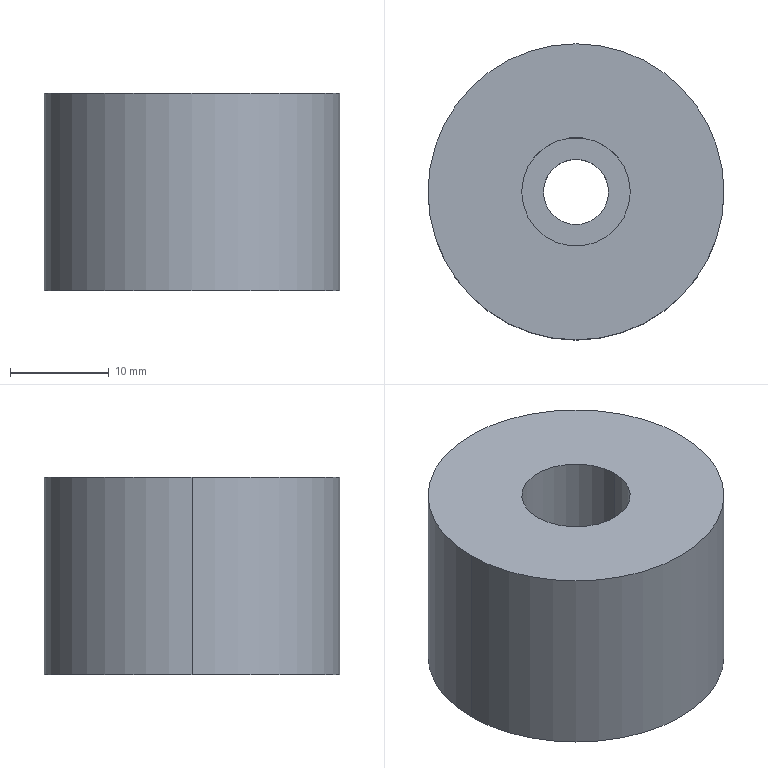Part | SolidWorks | features BaseBody 1 | 1 solid | 9 faces | box 30 x 30 x 20 mm | volume 12966 mm3 | cylinder 6 | plane 3 | commonest cylinder face diameters 6.6 x2 11 x2 30 x2
STEP:
#1=CARTESIAN_POINT('',(-15.,0.,20.));
#2=VERTEX_POINT('',#1);
#3=CARTESIAN_POINT('',(15.,0.,20.));
#4=VERTEX_POINT('',#3);
#5=CARTESIAN_POINT('',(0.,0.,20.));
#6=DIRECTION('',(0.,0.,-1.));
#7=DIRECTION('',(-1.,0.,0.));
#8=AXIS2_PLACEMENT_3D('',#5,#6,#7);
#9=CIRCLE('',#8,15.);
#10=EDGE_CURVE('',#2,#4,#9,.T.);
#11=ORIENTED_EDGE('',*,*,#10,.T.);
#12=CARTESIAN_POINT('',(15.,0.,0.));
#13=VERTEX_POINT('',#12);
#14=CARTESIAN_POINT('',(15.,0.,20.));
#15=DIRECTION('',(0.,0.,-1.));
#16=VECTOR('',#15,1000.);
#17=LINE('',#14,#16);
#18=EDGE_CURVE('',#4,#13,#17,.T.);
#19=ORIENTED_EDGE('',*,*,#18,.T.);
#20=CARTESIAN_POINT('',(-15.,0.,0.));
#21=VERTEX_POINT('',#20);
#22=CARTESIAN_POINT('',(0.,0.,0.));
#23=DIRECTION('',(0.,0.,1.));
#24=DIRECTION('',(-1.,0.,0.));
#25=AXIS2_PLACEMENT_3D('',#22,#23,#24);
#26=CIRCLE('',#25,15.);
#27=EDGE_CURVE('',#13,#21,#26,.T.);
#28=ORIENTED_EDGE('',*,*,#27,.T.);
#29=CARTESIAN_POINT('',(-15.,0.,20.));
#30=DIRECTION('',(0.,0.,-1.));
#31=VECTOR('',#30,1000.);
#32=LINE('',#29,#31);
#33=EDGE_CURVE('',#2,#21,#32,.T.);
#34=ORIENTED_EDGE('',*,*,#33,.F.);
#35=EDGE_LOOP('',(#11,#19,#28,#34));
#36=FACE_OUTER_BOUND('',#35,.T.);
#37=CARTESIAN_POINT('',(0.,0.,20.));
#38=DIRECTION('',(0.,0.,-1.));
#39=DIRECTION('',(-1.,0.,0.));
#40=AXIS2_PLACEMENT_3D('',#37,#38,#39);
#41=CYLINDRICAL_SURFACE('',#40,15.);
#42=ADVANCED_FACE('',(#36),#41,.T.);
#43=CARTESIAN_POINT('',(3.3,0.,0.));
#44=VERTEX_POINT('',#43);
#45=CARTESIAN_POINT('',(-3.3,0.,0.));
#46=VERTEX_POINT('',#45);
#47=CARTESIAN_POINT('',(0.,0.,0.));
#48=DIRECTION('',(0.,0.,-1.));
#49=DIRECTION('',(1.,0.,0.));
#50=AXIS2_PLACEMENT_3D('',#47,#48,#49);
#51=CIRCLE('',#50,3.3);
#52=EDGE_CURVE('',#44,#46,#51,.T.);
#53=ORIENTED_EDGE('',*,*,#52,.T.);
#54=CARTESIAN_POINT('',(-3.3,0.,12.));
#55=VERTEX_POINT('',#54);
#56=CARTESIAN_POINT('',(-3.3,0.,20.));
#57=DIRECTION('',(0.,0.,1.));
#58=VECTOR('',#57,1000.);
#59=LINE('',#56,#58);
#60=EDGE_CURVE('',#46,#55,#59,.T.);
#61=ORIENTED_EDGE('',*,*,#60,.T.);
#62=CARTESIAN_POINT('',(3.3,0.,12.));
#63=VERTEX_POINT('',#62);
#64=CARTESIAN_POINT('',(0.,0.,12.));
#65=DIRECTION('',(0.,0.,-1.));
#66=DIRECTION('',(1.,0.,0.));
#67=AXIS2_PLACEMENT_3D('',#64,#65,#66);
#68=CIRCLE('',#67,3.3);
#69=EDGE_CURVE('',#63,#55,#68,.T.);
#70=ORIENTED_EDGE('',*,*,#69,.F.);
#71=CARTESIAN_POINT('',(3.3,0.,20.));
#72=DIRECTION('',(0.,0.,1.));
#73=VECTOR('',#72,1000.);
#74=LINE('',#71,#73);
#75=EDGE_CURVE('',#44,#63,#74,.T.);
#76=ORIENTED_EDGE('',*,*,#75,.F.);
#77=EDGE_LOOP('',(#53,#61,#70,#76));
#78=FACE_OUTER_BOUND('',#77,.T.);
#79=CARTESIAN_POINT('',(0.,0.,20.));
#80=DIRECTION('',(0.,0.,1.));
#81=DIRECTION('',(1.,0.,0.));
#82=AXIS2_PLACEMENT_3D('',#79,#80,#81);
#83=CYLINDRICAL_SURFACE('',#82,3.3);
#84=ADVANCED_FACE('',(#78),#83,.F.);
#85=CARTESIAN_POINT('',(-5.5,0.,12.));
#86=VERTEX_POINT('',#85);
#87=CARTESIAN_POINT('',(5.5,0.,12.));
#88=VERTEX_POINT('',#87);
#89=CARTESIAN_POINT('',(0.,0.,12.));
#90=DIRECTION('',(0.,0.,1.));
#91=DIRECTION('',(1.,0.,0.));
#92=AXIS2_PLACEMENT_3D('',#89,#90,#91);
#93=CIRCLE('',#92,5.5);
#94=EDGE_CURVE('',#86,#88,#93,.T.);
#95=ORIENTED_EDGE('',*,*,#94,.F.);
#96=CARTESIAN_POINT('',(-5.5,0.,20.));
#97=VERTEX_POINT('',#96);
#98=CARTESIAN_POINT('',(-5.5,0.,20.));
#99=DIRECTION('',(0.,0.,1.));
#100=VECTOR('',#99,1000.);
#101=LINE('',#98,#100);
#102=EDGE_CURVE('',#86,#97,#101,.T.);
#103=ORIENTED_EDGE('',*,*,#102,.T.);
#104=CARTESIAN_POINT('',(5.5,0.,20.));
#105=VERTEX_POINT('',#104);
#106=CARTESIAN_POINT('',(0.,0.,20.));
#107=DIRECTION('',(0.,0.,-1.));
#108=DIRECTION('',(1.,0.,0.));
#109=AXIS2_PLACEMENT_3D('',#106,#107,#108);
#110=CIRCLE('',#109,5.5);
#111=EDGE_CURVE('',#105,#97,#110,.T.);
#112=ORIENTED_EDGE('',*,*,#111,.F.);
#113=CARTESIAN_POINT('',(5.5,0.,20.));
#114=DIRECTION('',(0.,0.,1.));
#115=VECTOR('',#114,1000.);
#116=LINE('',#113,#115);
#117=EDGE_CURVE('',#88,#105,#116,.T.);
#118=ORIENTED_EDGE('',*,*,#117,.F.);
#119=EDGE_LOOP('',(#95,#103,#112,#118));
#120=FACE_OUTER_BOUND('',#119,.T.);
#121=CARTESIAN_POINT('',(0.,0.,20.));
#122=DIRECTION('',(0.,0.,1.));
#123=DIRECTION('',(1.,0.,0.));
#124=AXIS2_PLACEMENT_3D('',#121,#122,#123);
#125=CYLINDRICAL_SURFACE('',#124,5.5);
#126=ADVANCED_FACE('',(#120),#125,.F.);
#127=ORIENTED_EDGE('',*,*,#18,.F.);
#128=CARTESIAN_POINT('',(0.,0.,20.));
#129=DIRECTION('',(0.,0.,-1.));
#130=DIRECTION('',(-1.,0.,0.));
#131=AXIS2_PLACEMENT_3D('',#128,#129,#130);
#132=CIRCLE('',#131,15.);
#133=EDGE_CURVE('',#4,#2,#132,.T.);
#134=ORIENTED_EDGE('',*,*,#133,.T.);
#135=ORIENTED_EDGE('',*,*,#33,.T.);
#136=CARTESIAN_POINT('',(0.,0.,0.));
#137=DIRECTION('',(0.,0.,1.));
#138=DIRECTION('',(-1.,0.,0.));
#139=AXIS2_PLACEMENT_3D('',#136,#137,#138);
#140=CIRCLE('',#139,15.);
#141=EDGE_CURVE('',#21,#13,#140,.T.);
#142=ORIENTED_EDGE('',*,*,#141,.T.);
#143=EDGE_LOOP('',(#127,#134,#135,#142));
#144=FACE_OUTER_BOUND('',#143,.T.);
#145=CARTESIAN_POINT('',(0.,0.,20.));
#146=DIRECTION('',(0.,0.,-1.));
#147=DIRECTION('',(-1.,0.,0.));
#148=AXIS2_PLACEMENT_3D('',#145,#146,#147);
#149=CYLINDRICAL_SURFACE('',#148,15.);
#150=ADVANCED_FACE('',(#144),#149,.T.);
#151=ORIENTED_EDGE('',*,*,#141,.F.);
#152=ORIENTED_EDGE('',*,*,#27,.F.);
#153=EDGE_LOOP('',(#151,#152));
#154=FACE_OUTER_BOUND('',#153,.T.);
#155=ORIENTED_EDGE('',*,*,#52,.F.);
#156=CARTESIAN_POINT('',(0.,0.,0.));
#157=DIRECTION('',(0.,0.,-1.));
#158=DIRECTION('',(1.,0.,0.));
#159=AXIS2_PLACEMENT_3D('',#156,#157,#158);
#160=CIRCLE('',#159,3.3);
#161=EDGE_CURVE('',#46,#44,#160,.T.);
#162=ORIENTED_EDGE('',*,*,#161,.F.);
#163=EDGE_LOOP('',(#155,#162));
#164=FACE_BOUND('',#163,.T.);
#165=CARTESIAN_POINT('',(0.,0.,0.));
#166=DIRECTION('',(0.,0.,1.));
#167=DIRECTION('',(1.,0.,0.));
#168=AXIS2_PLACEMENT_3D('',#165,#166,#167);
#169=PLANE('',#168);
#170=ADVANCED_FACE('',(#154,#164),#169,.F.);
#171=ORIENTED_EDGE('',*,*,#10,.F.);
#172=ORIENTED_EDGE('',*,*,#133,.F.);
#173=EDGE_LOOP('',(#171,#172));
#174=FACE_OUTER_BOUND('',#173,.T.);
#175=ORIENTED_EDGE('',*,*,#111,.T.);
#176=CARTESIAN_POINT('',(0.,0.,20.));
#177=DIRECTION('',(0.,0.,-1.));
#178=DIRECTION('',(1.,0.,0.));
#179=AXIS2_PLACEMENT_3D('',#176,#177,#178);
#180=CIRCLE('',#179,5.5);
#181=EDGE_CURVE('',#97,#105,#180,.T.);
#182=ORIENTED_EDGE('',*,*,#181,.T.);
#183=EDGE_LOOP('',(#175,#182));
#184=FACE_BOUND('',#183,.T.);
#185=CARTESIAN_POINT('',(0.,0.,20.));
#186=DIRECTION('',(0.,0.,1.));
#187=DIRECTION('',(1.,0.,0.));
#188=AXIS2_PLACEMENT_3D('',#185,#186,#187);
#189=PLANE('',#188);
#190=ADVANCED_FACE('',(#174,#184),#189,.T.);
#191=ORIENTED_EDGE('',*,*,#60,.F.);
#192=ORIENTED_EDGE('',*,*,#161,.T.);
#193=ORIENTED_EDGE('',*,*,#75,.T.);
#194=CARTESIAN_POINT('',(0.,0.,12.));
#195=DIRECTION('',(0.,0.,-1.));
#196=DIRECTION('',(1.,0.,0.));
#197=AXIS2_PLACEMENT_3D('',#194,#195,#196);
#198=CIRCLE('',#197,3.3);
#199=EDGE_CURVE('',#55,#63,#198,.T.);
#200=ORIENTED_EDGE('',*,*,#199,.F.);
#201=EDGE_LOOP('',(#191,#192,#193,#200));
#202=FACE_OUTER_BOUND('',#201,.T.);
#203=CARTESIAN_POINT('',(0.,0.,20.));
#204=DIRECTION('',(0.,0.,1.));
#205=DIRECTION('',(1.,0.,0.));
#206=AXIS2_PLACEMENT_3D('',#203,#204,#205);
#207=CYLINDRICAL_SURFACE('',#206,3.3);
#208=ADVANCED_FACE('',(#202),#207,.F.);
#209=ORIENTED_EDGE('',*,*,#102,.F.);
#210=CARTESIAN_POINT('',(0.,0.,12.));
#211=DIRECTION('',(0.,0.,1.));
#212=DIRECTION('',(1.,0.,0.));
#213=AXIS2_PLACEMENT_3D('',#210,#211,#212);
#214=CIRCLE('',#213,5.5);
#215=EDGE_CURVE('',#88,#86,#214,.T.);
#216=ORIENTED_EDGE('',*,*,#215,.F.);
#217=ORIENTED_EDGE('',*,*,#117,.T.);
#218=ORIENTED_EDGE('',*,*,#181,.F.);
#219=EDGE_LOOP('',(#209,#216,#217,#218));
#220=FACE_OUTER_BOUND('',#219,.T.);
#221=CARTESIAN_POINT('',(0.,0.,20.));
#222=DIRECTION('',(0.,0.,1.));
#223=DIRECTION('',(1.,0.,0.));
#224=AXIS2_PLACEMENT_3D('',#221,#222,#223);
#225=CYLINDRICAL_SURFACE('',#224,5.5);
#226=ADVANCED_FACE('',(#220),#225,.F.);
#227=ORIENTED_EDGE('',*,*,#215,.T.);
#228=ORIENTED_EDGE('',*,*,#94,.T.);
#229=EDGE_LOOP('',(#227,#228));
#230=FACE_OUTER_BOUND('',#229,.T.);
#231=ORIENTED_EDGE('',*,*,#69,.T.);
#232=ORIENTED_EDGE('',*,*,#199,.T.);
#233=EDGE_LOOP('',(#231,#232));
#234=FACE_BOUND('',#233,.T.);
#235=CARTESIAN_POINT('',(3.3,0.,12.));
#236=DIRECTION('',(0.,0.,-1.));
#237=DIRECTION('',(-1.,0.,0.));
#238=AXIS2_PLACEMENT_3D('',#235,#236,#237);
#239=PLANE('',#238);
#240=ADVANCED_FACE('',(#230,#234),#239,.F.);
#241=CLOSED_SHELL('',(#42,#84,#126,#150,#170,#190,#208,#226,#240));
#242=MANIFOLD_SOLID_BREP('',#241);
#243=CARTESIAN_POINT('',(0.,0.,0.));
#244=DIRECTION('',(0.,0.,1.));
#245=DIRECTION('',(1.,0.,0.));
#246=AXIS2_PLACEMENT_3D('',#243,#244,#245);
#247=(LENGTH_UNIT()NAMED_UNIT(*)SI_UNIT(.MILLI.,.METRE.));
#248=UNCERTAINTY_MEASURE_WITH_UNIT(LENGTH_MEASURE(0.00001),#247,'','');
#249=(NAMED_UNIT(*)PLANE_ANGLE_UNIT()SI_UNIT($,.RADIAN.));
#250=(NAMED_UNIT(*)SI_UNIT($,.STERADIAN.)SOLID_ANGLE_UNIT());
#251=(GEOMETRIC_REPRESENTATION_CONTEXT(3)GLOBAL_UNCERTAINTY_ASSIGNED_CONTEXT((#248))GLOBAL_UNIT_ASSIGNED_CONTEXT((#247,#249,#250))REPRESENTATION_CONTEXT('',''));
#252=ADVANCED_BREP_SHAPE_REPRESENTATION('',(#242,#246),#251);